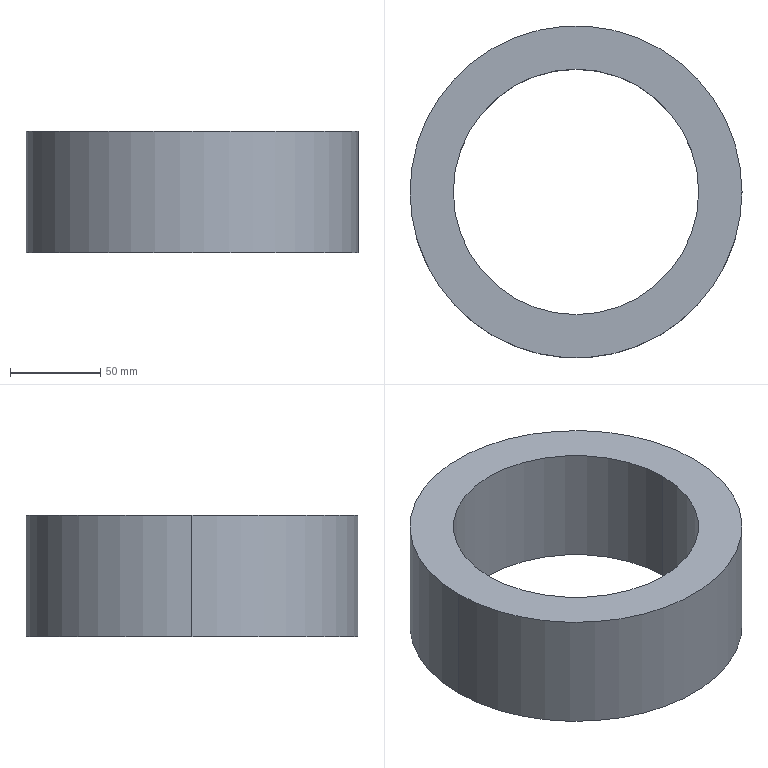Part | SolidWorks | features BaseBody 1 | 1 solid | 6 faces | box 184 x 184 x 67.2 mm | volume 810682 mm3 | cylinder 4 | plane 2 | commonest cylinder face diameters 136 x2 184 x2
STEP:
#1=CARTESIAN_POINT('',(197.077,953.249,657.507));
#2=VERTEX_POINT('',#1);
#3=CARTESIAN_POINT('',(197.077,953.249,724.707));
#4=VERTEX_POINT('',#3);
#5=CARTESIAN_POINT('',(197.077,953.249,657.507));
#6=DIRECTION('',(0.,0.,1.));
#7=VECTOR('',#6,1000.);
#8=LINE('',#5,#7);
#9=EDGE_CURVE('',#2,#4,#8,.T.);
#10=ORIENTED_EDGE('',*,*,#9,.F.);
#11=CARTESIAN_POINT('',(333.077,953.249,657.507));
#12=VERTEX_POINT('',#11);
#13=CARTESIAN_POINT('',(265.077,953.249,657.507));
#14=DIRECTION('',(0.,0.,1.));
#15=DIRECTION('',(1.,0.,0.));
#16=AXIS2_PLACEMENT_3D('',#13,#14,#15);
#17=CIRCLE('',#16,68.);
#18=EDGE_CURVE('',#12,#2,#17,.T.);
#19=ORIENTED_EDGE('',*,*,#18,.F.);
#20=CARTESIAN_POINT('',(333.077,953.249,724.707));
#21=VERTEX_POINT('',#20);
#22=CARTESIAN_POINT('',(333.077,953.249,657.507));
#23=DIRECTION('',(0.,0.,1.));
#24=VECTOR('',#23,1000.);
#25=LINE('',#22,#24);
#26=EDGE_CURVE('',#12,#21,#25,.T.);
#27=ORIENTED_EDGE('',*,*,#26,.T.);
#28=CARTESIAN_POINT('',(265.077,953.249,724.707));
#29=DIRECTION('',(0.,0.,1.));
#30=DIRECTION('',(1.,0.,0.));
#31=AXIS2_PLACEMENT_3D('',#28,#29,#30);
#32=CIRCLE('',#31,68.);
#33=EDGE_CURVE('',#21,#4,#32,.T.);
#34=ORIENTED_EDGE('',*,*,#33,.T.);
#35=EDGE_LOOP('',(#10,#19,#27,#34));
#36=FACE_OUTER_BOUND('',#35,.T.);
#37=CARTESIAN_POINT('',(265.077,953.249,657.507));
#38=DIRECTION('',(0.,0.,1.));
#39=DIRECTION('',(1.,0.,0.));
#40=AXIS2_PLACEMENT_3D('',#37,#38,#39);
#41=CYLINDRICAL_SURFACE('',#40,68.);
#42=ADVANCED_FACE('',(#36),#41,.F.);
#43=ORIENTED_EDGE('',*,*,#18,.T.);
#44=CARTESIAN_POINT('',(265.077,953.249,657.507));
#45=DIRECTION('',(0.,0.,1.));
#46=DIRECTION('',(1.,0.,0.));
#47=AXIS2_PLACEMENT_3D('',#44,#45,#46);
#48=CIRCLE('',#47,68.);
#49=EDGE_CURVE('',#2,#12,#48,.T.);
#50=ORIENTED_EDGE('',*,*,#49,.T.);
#51=EDGE_LOOP('',(#43,#50));
#52=FACE_BOUND('',#51,.T.);
#53=CARTESIAN_POINT('',(357.077,953.249,657.507));
#54=VERTEX_POINT('',#53);
#55=CARTESIAN_POINT('',(173.077,953.249,657.507));
#56=VERTEX_POINT('',#55);
#57=CARTESIAN_POINT('',(265.077,953.249,657.507));
#58=DIRECTION('',(0.,0.,1.));
#59=DIRECTION('',(1.,0.,0.));
#60=AXIS2_PLACEMENT_3D('',#57,#58,#59);
#61=CIRCLE('',#60,92.);
#62=EDGE_CURVE('',#54,#56,#61,.T.);
#63=ORIENTED_EDGE('',*,*,#62,.F.);
#64=CARTESIAN_POINT('',(265.077,953.249,657.507));
#65=DIRECTION('',(0.,0.,1.));
#66=DIRECTION('',(1.,0.,0.));
#67=AXIS2_PLACEMENT_3D('',#64,#65,#66);
#68=CIRCLE('',#67,92.);
#69=EDGE_CURVE('',#56,#54,#68,.T.);
#70=ORIENTED_EDGE('',*,*,#69,.F.);
#71=EDGE_LOOP('',(#63,#70));
#72=FACE_OUTER_BOUND('',#71,.T.);
#73=CARTESIAN_POINT('',(357.077,953.249,657.507));
#74=DIRECTION('',(0.,0.,-1.));
#75=DIRECTION('',(0.,-1.,0.));
#76=AXIS2_PLACEMENT_3D('',#73,#74,#75);
#77=PLANE('',#76);
#78=ADVANCED_FACE('',(#52,#72),#77,.T.);
#79=CARTESIAN_POINT('',(173.077,953.249,724.707));
#80=VERTEX_POINT('',#79);
#81=CARTESIAN_POINT('',(173.077,953.249,657.507));
#82=DIRECTION('',(0.,0.,1.));
#83=VECTOR('',#82,1000.);
#84=LINE('',#81,#83);
#85=EDGE_CURVE('',#56,#80,#84,.T.);
#86=ORIENTED_EDGE('',*,*,#85,.F.);
#87=ORIENTED_EDGE('',*,*,#69,.T.);
#88=CARTESIAN_POINT('',(357.077,953.249,724.707));
#89=VERTEX_POINT('',#88);
#90=CARTESIAN_POINT('',(357.077,953.249,657.507));
#91=DIRECTION('',(0.,0.,1.));
#92=VECTOR('',#91,1000.);
#93=LINE('',#90,#92);
#94=EDGE_CURVE('',#54,#89,#93,.T.);
#95=ORIENTED_EDGE('',*,*,#94,.T.);
#96=CARTESIAN_POINT('',(265.077,953.249,724.707));
#97=DIRECTION('',(0.,0.,1.));
#98=DIRECTION('',(1.,0.,0.));
#99=AXIS2_PLACEMENT_3D('',#96,#97,#98);
#100=CIRCLE('',#99,92.);
#101=EDGE_CURVE('',#80,#89,#100,.T.);
#102=ORIENTED_EDGE('',*,*,#101,.F.);
#103=EDGE_LOOP('',(#86,#87,#95,#102));
#104=FACE_OUTER_BOUND('',#103,.T.);
#105=CARTESIAN_POINT('',(265.077,953.249,657.507));
#106=DIRECTION('',(0.,0.,1.));
#107=DIRECTION('',(1.,0.,0.));
#108=AXIS2_PLACEMENT_3D('',#105,#106,#107);
#109=CYLINDRICAL_SURFACE('',#108,92.);
#110=ADVANCED_FACE('',(#104),#109,.T.);
#111=ORIENTED_EDGE('',*,*,#33,.F.);
#112=CARTESIAN_POINT('',(265.077,953.249,724.707));
#113=DIRECTION('',(0.,0.,1.));
#114=DIRECTION('',(1.,0.,0.));
#115=AXIS2_PLACEMENT_3D('',#112,#113,#114);
#116=CIRCLE('',#115,68.);
#117=EDGE_CURVE('',#4,#21,#116,.T.);
#118=ORIENTED_EDGE('',*,*,#117,.F.);
#119=EDGE_LOOP('',(#111,#118));
#120=FACE_BOUND('',#119,.T.);
#121=CARTESIAN_POINT('',(265.077,953.249,724.707));
#122=DIRECTION('',(0.,0.,1.));
#123=DIRECTION('',(1.,0.,0.));
#124=AXIS2_PLACEMENT_3D('',#121,#122,#123);
#125=CIRCLE('',#124,92.);
#126=EDGE_CURVE('',#89,#80,#125,.T.);
#127=ORIENTED_EDGE('',*,*,#126,.T.);
#128=ORIENTED_EDGE('',*,*,#101,.T.);
#129=EDGE_LOOP('',(#127,#128));
#130=FACE_OUTER_BOUND('',#129,.T.);
#131=CARTESIAN_POINT('',(333.077,953.249,724.707));
#132=DIRECTION('',(0.,0.,1.));
#133=DIRECTION('',(1.,0.,0.));
#134=AXIS2_PLACEMENT_3D('',#131,#132,#133);
#135=PLANE('',#134);
#136=ADVANCED_FACE('',(#120,#130),#135,.T.);
#137=ORIENTED_EDGE('',*,*,#62,.T.);
#138=ORIENTED_EDGE('',*,*,#85,.T.);
#139=ORIENTED_EDGE('',*,*,#126,.F.);
#140=ORIENTED_EDGE('',*,*,#94,.F.);
#141=EDGE_LOOP('',(#137,#138,#139,#140));
#142=FACE_OUTER_BOUND('',#141,.T.);
#143=CARTESIAN_POINT('',(265.077,953.249,657.507));
#144=DIRECTION('',(0.,0.,1.));
#145=DIRECTION('',(1.,0.,0.));
#146=AXIS2_PLACEMENT_3D('',#143,#144,#145);
#147=CYLINDRICAL_SURFACE('',#146,92.);
#148=ADVANCED_FACE('',(#142),#147,.T.);
#149=ORIENTED_EDGE('',*,*,#49,.F.);
#150=ORIENTED_EDGE('',*,*,#9,.T.);
#151=ORIENTED_EDGE('',*,*,#117,.T.);
#152=ORIENTED_EDGE('',*,*,#26,.F.);
#153=EDGE_LOOP('',(#149,#150,#151,#152));
#154=FACE_OUTER_BOUND('',#153,.T.);
#155=CARTESIAN_POINT('',(265.077,953.249,657.507));
#156=DIRECTION('',(0.,0.,1.));
#157=DIRECTION('',(1.,0.,0.));
#158=AXIS2_PLACEMENT_3D('',#155,#156,#157);
#159=CYLINDRICAL_SURFACE('',#158,68.);
#160=ADVANCED_FACE('',(#154),#159,.F.);
#161=CLOSED_SHELL('',(#42,#78,#110,#136,#148,#160));
#162=MANIFOLD_SOLID_BREP('',#161);
#163=CARTESIAN_POINT('',(0.,0.,0.));
#164=DIRECTION('',(0.,0.,1.));
#165=DIRECTION('',(1.,0.,0.));
#166=AXIS2_PLACEMENT_3D('',#163,#164,#165);
#167=(LENGTH_UNIT()NAMED_UNIT(*)SI_UNIT(.MILLI.,.METRE.));
#168=UNCERTAINTY_MEASURE_WITH_UNIT(LENGTH_MEASURE(0.00001),#167,'','');
#169=(NAMED_UNIT(*)PLANE_ANGLE_UNIT()SI_UNIT($,.RADIAN.));
#170=(NAMED_UNIT(*)SI_UNIT($,.STERADIAN.)SOLID_ANGLE_UNIT());
#171=(GEOMETRIC_REPRESENTATION_CONTEXT(3)GLOBAL_UNCERTAINTY_ASSIGNED_CONTEXT((#168))GLOBAL_UNIT_ASSIGNED_CONTEXT((#167,#169,#170))REPRESENTATION_CONTEXT('',''));
#172=ADVANCED_BREP_SHAPE_REPRESENTATION('',(#162,#166),#171);